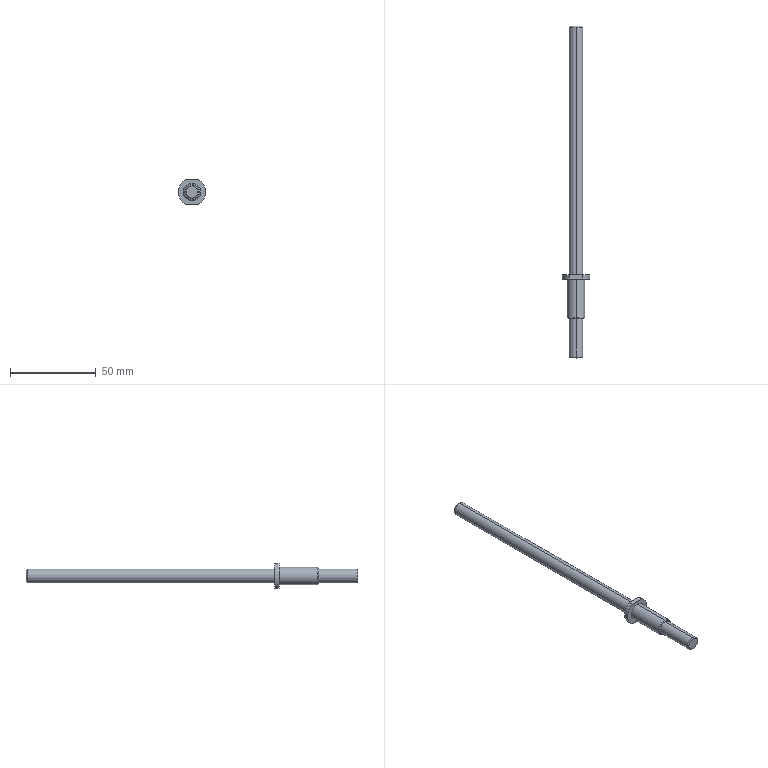Part | STEP file | 11-FG-B04411 | 1 solid | 21 faces | box 16 x 193.5 x 14 mm | volume 10709 mm3 | cylinder 8 | plane 7 | cone 6 | commonest cylinder face diameters 8 x4 10 x2 16 x2
STEP:
#1=CARTESIAN_POINT('',(0.,193.5,3.));
#2=VERTEX_POINT('',#1);
#3=CARTESIAN_POINT('',(0.,193.5,-3.));
#4=VERTEX_POINT('',#3);
#5=CARTESIAN_POINT('',(0.,193.5,0.));
#6=DIRECTION('',(0.,1.,0.));
#7=DIRECTION('',(0.,0.,1.));
#8=AXIS2_PLACEMENT_3D('',#5,#6,#7);
#9=CIRCLE('',#8,3.);
#10=EDGE_CURVE('',#2,#4,#9,.T.);
#11=ORIENTED_EDGE('',*,*,#10,.F.);
#12=CARTESIAN_POINT('',(0.,192.5,4.));
#13=VERTEX_POINT('',#12);
#14=CARTESIAN_POINT('',(0.,192.5,4.));
#15=DIRECTION('',(0.,-0.7071,0.7071));
#16=VECTOR('',#15,1000.);
#17=LINE('',#14,#16);
#18=EDGE_CURVE('',#2,#13,#17,.T.);
#19=ORIENTED_EDGE('',*,*,#18,.T.);
#20=CARTESIAN_POINT('',(0.,192.5,-4.));
#21=VERTEX_POINT('',#20);
#22=CARTESIAN_POINT('',(0.,192.5,0.));
#23=DIRECTION('',(0.,-1.,0.));
#24=DIRECTION('',(0.,0.,1.));
#25=AXIS2_PLACEMENT_3D('',#22,#23,#24);
#26=CIRCLE('',#25,4.);
#27=EDGE_CURVE('',#21,#13,#26,.T.);
#28=ORIENTED_EDGE('',*,*,#27,.F.);
#29=CARTESIAN_POINT('',(0.,192.5,-4.));
#30=DIRECTION('',(0.,-0.7071,-0.7071));
#31=VECTOR('',#30,1000.);
#32=LINE('',#29,#31);
#33=EDGE_CURVE('',#4,#21,#32,.T.);
#34=ORIENTED_EDGE('',*,*,#33,.F.);
#35=EDGE_LOOP('',(#11,#19,#28,#34));
#36=FACE_OUTER_BOUND('',#35,.T.);
#37=CARTESIAN_POINT('',(0.,192.5,0.));
#38=DIRECTION('',(0.,-1.,0.));
#39=DIRECTION('',(0.,0.,-1.));
#40=AXIS2_PLACEMENT_3D('',#37,#38,#39);
#41=CONICAL_SURFACE('',#40,4.,0.7854);
#42=ADVANCED_FACE('',(#36),#41,.T.);
#43=CARTESIAN_POINT('',(0.,23.,-4.5));
#44=VERTEX_POINT('',#43);
#45=CARTESIAN_POINT('',(0.,23.,4.5));
#46=VERTEX_POINT('',#45);
#47=CARTESIAN_POINT('',(0.,23.,0.));
#48=DIRECTION('',(0.,-1.,0.));
#49=DIRECTION('',(0.,0.,-1.));
#50=AXIS2_PLACEMENT_3D('',#47,#48,#49);
#51=CIRCLE('',#50,4.5);
#52=EDGE_CURVE('',#44,#46,#51,.T.);
#53=ORIENTED_EDGE('',*,*,#52,.F.);
#54=CARTESIAN_POINT('',(0.,23.5,-5.));
#55=VERTEX_POINT('',#54);
#56=CARTESIAN_POINT('',(0.,23.,-4.5));
#57=DIRECTION('',(0.,0.7071,-0.7071));
#58=VECTOR('',#57,1000.);
#59=LINE('',#56,#58);
#60=EDGE_CURVE('',#44,#55,#59,.T.);
#61=ORIENTED_EDGE('',*,*,#60,.T.);
#62=CARTESIAN_POINT('',(0.,23.5,5.));
#63=VERTEX_POINT('',#62);
#64=CARTESIAN_POINT('',(0.,23.5,0.));
#65=DIRECTION('',(0.,1.,0.));
#66=DIRECTION('',(0.,0.,-1.));
#67=AXIS2_PLACEMENT_3D('',#64,#65,#66);
#68=CIRCLE('',#67,5.);
#69=EDGE_CURVE('',#63,#55,#68,.T.);
#70=ORIENTED_EDGE('',*,*,#69,.F.);
#71=CARTESIAN_POINT('',(0.,23.,4.5));
#72=DIRECTION('',(0.,0.7071,0.7071));
#73=VECTOR('',#72,1000.);
#74=LINE('',#71,#73);
#75=EDGE_CURVE('',#46,#63,#74,.T.);
#76=ORIENTED_EDGE('',*,*,#75,.F.);
#77=EDGE_LOOP('',(#53,#61,#70,#76));
#78=FACE_OUTER_BOUND('',#77,.T.);
#79=CARTESIAN_POINT('',(0.,23.,0.));
#80=DIRECTION('',(0.,1.,0.));
#81=DIRECTION('',(0.,0.,1.));
#82=AXIS2_PLACEMENT_3D('',#79,#80,#81);
#83=CONICAL_SURFACE('',#82,4.5,0.7854);
#84=ADVANCED_FACE('',(#78),#83,.T.);
#85=CARTESIAN_POINT('',(0.,0.,-3.5));
#86=VERTEX_POINT('',#85);
#87=CARTESIAN_POINT('',(0.,0.,3.5));
#88=VERTEX_POINT('',#87);
#89=CARTESIAN_POINT('',(0.,0.,0.));
#90=DIRECTION('',(0.,-1.,0.));
#91=DIRECTION('',(0.,0.,-1.));
#92=AXIS2_PLACEMENT_3D('',#89,#90,#91);
#93=CIRCLE('',#92,3.5);
#94=EDGE_CURVE('',#86,#88,#93,.T.);
#95=ORIENTED_EDGE('',*,*,#94,.F.);
#96=CARTESIAN_POINT('',(0.,0.5,-4.));
#97=VERTEX_POINT('',#96);
#98=CARTESIAN_POINT('',(0.,0.,-3.5));
#99=DIRECTION('',(0.,0.7071,-0.7071));
#100=VECTOR('',#99,1000.);
#101=LINE('',#98,#100);
#102=EDGE_CURVE('',#86,#97,#101,.T.);
#103=ORIENTED_EDGE('',*,*,#102,.T.);
#104=CARTESIAN_POINT('',(0.,0.5,4.));
#105=VERTEX_POINT('',#104);
#106=CARTESIAN_POINT('',(0.,0.5,0.));
#107=DIRECTION('',(0.,1.,0.));
#108=DIRECTION('',(0.,0.,-1.));
#109=AXIS2_PLACEMENT_3D('',#106,#107,#108);
#110=CIRCLE('',#109,4.);
#111=EDGE_CURVE('',#105,#97,#110,.T.);
#112=ORIENTED_EDGE('',*,*,#111,.F.);
#113=CARTESIAN_POINT('',(0.,0.,3.5));
#114=DIRECTION('',(0.,0.7071,0.7071));
#115=VECTOR('',#114,1000.);
#116=LINE('',#113,#115);
#117=EDGE_CURVE('',#88,#105,#116,.T.);
#118=ORIENTED_EDGE('',*,*,#117,.F.);
#119=EDGE_LOOP('',(#95,#103,#112,#118));
#120=FACE_OUTER_BOUND('',#119,.T.);
#121=CARTESIAN_POINT('',(0.,0.,0.));
#122=DIRECTION('',(0.,1.,0.));
#123=DIRECTION('',(0.,0.,1.));
#124=AXIS2_PLACEMENT_3D('',#121,#122,#123);
#125=CONICAL_SURFACE('',#124,3.5,0.7854);
#126=ADVANCED_FACE('',(#120),#125,.T.);
#127=CARTESIAN_POINT('',(0.,23.,-4.));
#128=VERTEX_POINT('',#127);
#129=CARTESIAN_POINT('',(0.,23.,4.));
#130=VERTEX_POINT('',#129);
#131=CARTESIAN_POINT('',(0.,23.,0.));
#132=DIRECTION('',(0.,-1.,0.));
#133=DIRECTION('',(0.,0.,-1.));
#134=AXIS2_PLACEMENT_3D('',#131,#132,#133);
#135=CIRCLE('',#134,4.);
#136=EDGE_CURVE('',#128,#130,#135,.T.);
#137=ORIENTED_EDGE('',*,*,#136,.T.);
#138=CARTESIAN_POINT('',(0.,0.,4.));
#139=DIRECTION('',(0.,-1.,0.));
#140=VECTOR('',#139,1000.);
#141=LINE('',#138,#140);
#142=EDGE_CURVE('',#130,#105,#141,.T.);
#143=ORIENTED_EDGE('',*,*,#142,.T.);
#144=ORIENTED_EDGE('',*,*,#111,.T.);
#145=CARTESIAN_POINT('',(0.,0.,-4.));
#146=DIRECTION('',(0.,-1.,0.));
#147=VECTOR('',#146,1000.);
#148=LINE('',#145,#147);
#149=EDGE_CURVE('',#128,#97,#148,.T.);
#150=ORIENTED_EDGE('',*,*,#149,.F.);
#151=EDGE_LOOP('',(#137,#143,#144,#150));
#152=FACE_OUTER_BOUND('',#151,.T.);
#153=CARTESIAN_POINT('',(0.,0.,0.));
#154=DIRECTION('',(0.,-1.,0.));
#155=DIRECTION('',(0.,0.,-1.));
#156=AXIS2_PLACEMENT_3D('',#153,#154,#155);
#157=CYLINDRICAL_SURFACE('',#156,4.);
#158=ADVANCED_FACE('',(#152),#157,.T.);
#159=CARTESIAN_POINT('',(0.,46.,-5.));
#160=VERTEX_POINT('',#159);
#161=CARTESIAN_POINT('',(0.,46.,5.));
#162=VERTEX_POINT('',#161);
#163=CARTESIAN_POINT('',(0.,46.,0.));
#164=DIRECTION('',(0.,-1.,0.));
#165=DIRECTION('',(0.,0.,-1.));
#166=AXIS2_PLACEMENT_3D('',#163,#164,#165);
#167=CIRCLE('',#166,5.);
#168=EDGE_CURVE('',#160,#162,#167,.T.);
#169=ORIENTED_EDGE('',*,*,#168,.T.);
#170=CARTESIAN_POINT('',(0.,0.,5.));
#171=DIRECTION('',(0.,-1.,0.));
#172=VECTOR('',#171,1000.);
#173=LINE('',#170,#172);
#174=EDGE_CURVE('',#162,#63,#173,.T.);
#175=ORIENTED_EDGE('',*,*,#174,.T.);
#176=ORIENTED_EDGE('',*,*,#69,.T.);
#177=CARTESIAN_POINT('',(0.,0.,-5.));
#178=DIRECTION('',(0.,-1.,0.));
#179=VECTOR('',#178,1000.);
#180=LINE('',#177,#179);
#181=EDGE_CURVE('',#160,#55,#180,.T.);
#182=ORIENTED_EDGE('',*,*,#181,.F.);
#183=EDGE_LOOP('',(#169,#175,#176,#182));
#184=FACE_OUTER_BOUND('',#183,.T.);
#185=CARTESIAN_POINT('',(0.,0.,0.));
#186=DIRECTION('',(0.,-1.,0.));
#187=DIRECTION('',(0.,0.,-1.));
#188=AXIS2_PLACEMENT_3D('',#185,#186,#187);
#189=CYLINDRICAL_SURFACE('',#188,5.);
#190=ADVANCED_FACE('',(#184),#189,.T.);
#191=ORIENTED_EDGE('',*,*,#27,.T.);
#192=CARTESIAN_POINT('',(0.,48.5,4.));
#193=VERTEX_POINT('',#192);
#194=CARTESIAN_POINT('',(0.,0.,4.));
#195=DIRECTION('',(0.,-1.,0.));
#196=VECTOR('',#195,1000.);
#197=LINE('',#194,#196);
#198=EDGE_CURVE('',#13,#193,#197,.T.);
#199=ORIENTED_EDGE('',*,*,#198,.T.);
#200=CARTESIAN_POINT('',(0.,48.5,-4.));
#201=VERTEX_POINT('',#200);
#202=CARTESIAN_POINT('',(0.,48.5,0.));
#203=DIRECTION('',(0.,-1.,0.));
#204=DIRECTION('',(0.,0.,-1.));
#205=AXIS2_PLACEMENT_3D('',#202,#203,#204);
#206=CIRCLE('',#205,4.);
#207=EDGE_CURVE('',#201,#193,#206,.T.);
#208=ORIENTED_EDGE('',*,*,#207,.F.);
#209=CARTESIAN_POINT('',(0.,0.,-4.));
#210=DIRECTION('',(0.,-1.,0.));
#211=VECTOR('',#210,1000.);
#212=LINE('',#209,#211);
#213=EDGE_CURVE('',#21,#201,#212,.T.);
#214=ORIENTED_EDGE('',*,*,#213,.F.);
#215=EDGE_LOOP('',(#191,#199,#208,#214));
#216=FACE_OUTER_BOUND('',#215,.T.);
#217=CARTESIAN_POINT('',(0.,0.,0.));
#218=DIRECTION('',(0.,-1.,0.));
#219=DIRECTION('',(0.,0.,-1.));
#220=AXIS2_PLACEMENT_3D('',#217,#218,#219);
#221=CYLINDRICAL_SURFACE('',#220,4.);
#222=ADVANCED_FACE('',(#216),#221,.T.);
#223=CARTESIAN_POINT('',(3.873,46.,7.));
#224=VERTEX_POINT('',#223);
#225=CARTESIAN_POINT('',(3.873,48.5,7.));
#226=VERTEX_POINT('',#225);
#227=CARTESIAN_POINT('',(3.873,38.5,7.));
#228=DIRECTION('',(0.,1.,0.));
#229=VECTOR('',#228,1000.);
#230=LINE('',#227,#229);
#231=EDGE_CURVE('',#224,#226,#230,.T.);
#232=ORIENTED_EDGE('',*,*,#231,.F.);
#233=CARTESIAN_POINT('',(3.873,46.,-7.));
#234=VERTEX_POINT('',#233);
#235=CARTESIAN_POINT('',(0.,46.,0.));
#236=DIRECTION('',(0.,-1.,0.));
#237=DIRECTION('',(0.,0.,-1.));
#238=AXIS2_PLACEMENT_3D('',#235,#236,#237);
#239=CIRCLE('',#238,8.);
#240=EDGE_CURVE('',#234,#224,#239,.T.);
#241=ORIENTED_EDGE('',*,*,#240,.F.);
#242=CARTESIAN_POINT('',(3.873,48.5,-7.));
#243=VERTEX_POINT('',#242);
#244=CARTESIAN_POINT('',(3.873,38.5,-7.));
#245=DIRECTION('',(0.,1.,0.));
#246=VECTOR('',#245,1000.);
#247=LINE('',#244,#246);
#248=EDGE_CURVE('',#234,#243,#247,.T.);
#249=ORIENTED_EDGE('',*,*,#248,.T.);
#250=CARTESIAN_POINT('',(0.,48.5,0.));
#251=DIRECTION('',(0.,-1.,0.));
#252=DIRECTION('',(0.,0.,-1.));
#253=AXIS2_PLACEMENT_3D('',#250,#251,#252);
#254=CIRCLE('',#253,8.);
#255=EDGE_CURVE('',#243,#226,#254,.T.);
#256=ORIENTED_EDGE('',*,*,#255,.T.);
#257=EDGE_LOOP('',(#232,#241,#249,#256));
#258=FACE_OUTER_BOUND('',#257,.T.);
#259=CARTESIAN_POINT('',(0.,0.,0.));
#260=DIRECTION('',(0.,-1.,0.));
#261=DIRECTION('',(0.,0.,-1.));
#262=AXIS2_PLACEMENT_3D('',#259,#260,#261);
#263=CYLINDRICAL_SURFACE('',#262,8.);
#264=ADVANCED_FACE('',(#258),#263,.T.);
#265=CARTESIAN_POINT('',(0.,193.5,0.));
#266=DIRECTION('',(0.,1.,0.));
#267=DIRECTION('',(0.,0.,1.));
#268=AXIS2_PLACEMENT_3D('',#265,#266,#267);
#269=CIRCLE('',#268,3.);
#270=EDGE_CURVE('',#4,#2,#269,.T.);
#271=ORIENTED_EDGE('',*,*,#270,.T.);
#272=ORIENTED_EDGE('',*,*,#10,.T.);
#273=EDGE_LOOP('',(#271,#272));
#274=FACE_OUTER_BOUND('',#273,.T.);
#275=CARTESIAN_POINT('',(0.,193.5,0.));
#276=DIRECTION('',(0.,1.,0.));
#277=DIRECTION('',(0.,0.,1.));
#278=AXIS2_PLACEMENT_3D('',#275,#276,#277);
#279=PLANE('',#278);
#280=ADVANCED_FACE('',(#274),#279,.T.);
#281=ORIENTED_EDGE('',*,*,#198,.F.);
#282=CARTESIAN_POINT('',(0.,192.5,0.));
#283=DIRECTION('',(0.,-1.,0.));
#284=DIRECTION('',(0.,0.,1.));
#285=AXIS2_PLACEMENT_3D('',#282,#283,#284);
#286=CIRCLE('',#285,4.);
#287=EDGE_CURVE('',#13,#21,#286,.T.);
#288=ORIENTED_EDGE('',*,*,#287,.T.);
#289=ORIENTED_EDGE('',*,*,#213,.T.);
#290=CARTESIAN_POINT('',(0.,48.5,0.));
#291=DIRECTION('',(0.,-1.,0.));
#292=DIRECTION('',(0.,0.,-1.));
#293=AXIS2_PLACEMENT_3D('',#290,#291,#292);
#294=CIRCLE('',#293,4.);
#295=EDGE_CURVE('',#193,#201,#294,.T.);
#296=ORIENTED_EDGE('',*,*,#295,.F.);
#297=EDGE_LOOP('',(#281,#288,#289,#296));
#298=FACE_OUTER_BOUND('',#297,.T.);
#299=CARTESIAN_POINT('',(0.,0.,0.));
#300=DIRECTION('',(0.,-1.,0.));
#301=DIRECTION('',(0.,0.,-1.));
#302=AXIS2_PLACEMENT_3D('',#299,#300,#301);
#303=CYLINDRICAL_SURFACE('',#302,4.);
#304=ADVANCED_FACE('',(#298),#303,.T.);
#305=CARTESIAN_POINT('',(-3.873,48.5,7.));
#306=VERTEX_POINT('',#305);
#307=CARTESIAN_POINT('',(-3.873,48.5,7.));
#308=DIRECTION('',(-1.,0.,0.));
#309=VECTOR('',#308,1000.);
#310=LINE('',#307,#309);
#311=EDGE_CURVE('',#226,#306,#310,.T.);
#312=ORIENTED_EDGE('',*,*,#311,.F.);
#313=ORIENTED_EDGE('',*,*,#255,.F.);
#314=CARTESIAN_POINT('',(-3.873,48.5,-7.));
#315=VERTEX_POINT('',#314);
#316=CARTESIAN_POINT('',(-3.873,48.5,-7.));
#317=DIRECTION('',(1.,0.,0.));
#318=VECTOR('',#317,1000.);
#319=LINE('',#316,#318);
#320=EDGE_CURVE('',#315,#243,#319,.T.);
#321=ORIENTED_EDGE('',*,*,#320,.F.);
#322=CARTESIAN_POINT('',(0.,48.5,0.));
#323=DIRECTION('',(0.,-1.,0.));
#324=DIRECTION('',(0.,0.,-1.));
#325=AXIS2_PLACEMENT_3D('',#322,#323,#324);
#326=CIRCLE('',#325,8.);
#327=EDGE_CURVE('',#306,#315,#326,.T.);
#328=ORIENTED_EDGE('',*,*,#327,.F.);
#329=EDGE_LOOP('',(#312,#313,#321,#328));
#330=FACE_OUTER_BOUND('',#329,.T.);
#331=ORIENTED_EDGE('',*,*,#207,.T.);
#332=ORIENTED_EDGE('',*,*,#295,.T.);
#333=EDGE_LOOP('',(#331,#332));
#334=FACE_BOUND('',#333,.T.);
#335=CARTESIAN_POINT('',(4.,48.5,0.));
#336=DIRECTION('',(0.,1.,0.));
#337=DIRECTION('',(0.,0.,1.));
#338=AXIS2_PLACEMENT_3D('',#335,#336,#337);
#339=PLANE('',#338);
#340=ADVANCED_FACE('',(#330,#334),#339,.T.);
#341=CARTESIAN_POINT('',(-3.873,46.,7.));
#342=VERTEX_POINT('',#341);
#343=CARTESIAN_POINT('',(-3.873,38.5,7.));
#344=DIRECTION('',(0.,1.,0.));
#345=VECTOR('',#344,1000.);
#346=LINE('',#343,#345);
#347=EDGE_CURVE('',#342,#306,#346,.T.);
#348=ORIENTED_EDGE('',*,*,#347,.T.);
#349=ORIENTED_EDGE('',*,*,#327,.T.);
#350=CARTESIAN_POINT('',(-3.873,46.,-7.));
#351=VERTEX_POINT('',#350);
#352=CARTESIAN_POINT('',(-3.873,38.5,-7.));
#353=DIRECTION('',(0.,1.,0.));
#354=VECTOR('',#353,1000.);
#355=LINE('',#352,#354);
#356=EDGE_CURVE('',#351,#315,#355,.T.);
#357=ORIENTED_EDGE('',*,*,#356,.F.);
#358=CARTESIAN_POINT('',(0.,46.,0.));
#359=DIRECTION('',(0.,-1.,0.));
#360=DIRECTION('',(0.,0.,-1.));
#361=AXIS2_PLACEMENT_3D('',#358,#359,#360);
#362=CIRCLE('',#361,8.);
#363=EDGE_CURVE('',#342,#351,#362,.T.);
#364=ORIENTED_EDGE('',*,*,#363,.F.);
#365=EDGE_LOOP('',(#348,#349,#357,#364));
#366=FACE_OUTER_BOUND('',#365,.T.);
#367=CARTESIAN_POINT('',(0.,0.,0.));
#368=DIRECTION('',(0.,-1.,0.));
#369=DIRECTION('',(0.,0.,-1.));
#370=AXIS2_PLACEMENT_3D('',#367,#368,#369);
#371=CYLINDRICAL_SURFACE('',#370,8.);
#372=ADVANCED_FACE('',(#366),#371,.T.);
#373=CARTESIAN_POINT('',(8.,46.,7.));
#374=DIRECTION('',(1.,0.,0.));
#375=VECTOR('',#374,1000.);
#376=LINE('',#373,#375);
#377=EDGE_CURVE('',#342,#224,#376,.T.);
#378=ORIENTED_EDGE('',*,*,#377,.F.);
#379=ORIENTED_EDGE('',*,*,#363,.T.);
#380=CARTESIAN_POINT('',(8.,46.,-7.));
#381=DIRECTION('',(-1.,0.,0.));
#382=VECTOR('',#381,1000.);
#383=LINE('',#380,#382);
#384=EDGE_CURVE('',#234,#351,#383,.T.);
#385=ORIENTED_EDGE('',*,*,#384,.F.);
#386=ORIENTED_EDGE('',*,*,#240,.T.);
#387=EDGE_LOOP('',(#378,#379,#385,#386));
#388=FACE_OUTER_BOUND('',#387,.T.);
#389=ORIENTED_EDGE('',*,*,#168,.F.);
#390=CARTESIAN_POINT('',(0.,46.,0.));
#391=DIRECTION('',(0.,-1.,0.));
#392=DIRECTION('',(0.,0.,-1.));
#393=AXIS2_PLACEMENT_3D('',#390,#391,#392);
#394=CIRCLE('',#393,5.);
#395=EDGE_CURVE('',#162,#160,#394,.T.);
#396=ORIENTED_EDGE('',*,*,#395,.F.);
#397=EDGE_LOOP('',(#389,#396));
#398=FACE_BOUND('',#397,.T.);
#399=CARTESIAN_POINT('',(8.,46.,0.));
#400=DIRECTION('',(0.,-1.,0.));
#401=DIRECTION('',(0.,0.,-1.));
#402=AXIS2_PLACEMENT_3D('',#399,#400,#401);
#403=PLANE('',#402);
#404=ADVANCED_FACE('',(#388,#398),#403,.T.);
#405=ORIENTED_EDGE('',*,*,#174,.F.);
#406=ORIENTED_EDGE('',*,*,#395,.T.);
#407=ORIENTED_EDGE('',*,*,#181,.T.);
#408=CARTESIAN_POINT('',(0.,23.5,0.));
#409=DIRECTION('',(0.,1.,0.));
#410=DIRECTION('',(0.,0.,-1.));
#411=AXIS2_PLACEMENT_3D('',#408,#409,#410);
#412=CIRCLE('',#411,5.);
#413=EDGE_CURVE('',#55,#63,#412,.T.);
#414=ORIENTED_EDGE('',*,*,#413,.T.);
#415=EDGE_LOOP('',(#405,#406,#407,#414));
#416=FACE_OUTER_BOUND('',#415,.T.);
#417=CARTESIAN_POINT('',(0.,0.,0.));
#418=DIRECTION('',(0.,-1.,0.));
#419=DIRECTION('',(0.,0.,-1.));
#420=AXIS2_PLACEMENT_3D('',#417,#418,#419);
#421=CYLINDRICAL_SURFACE('',#420,5.);
#422=ADVANCED_FACE('',(#416),#421,.T.);
#423=CARTESIAN_POINT('',(0.,23.,0.));
#424=DIRECTION('',(0.,-1.,0.));
#425=DIRECTION('',(0.,0.,-1.));
#426=AXIS2_PLACEMENT_3D('',#423,#424,#425);
#427=CIRCLE('',#426,4.5);
#428=EDGE_CURVE('',#46,#44,#427,.T.);
#429=ORIENTED_EDGE('',*,*,#428,.T.);
#430=ORIENTED_EDGE('',*,*,#52,.T.);
#431=EDGE_LOOP('',(#429,#430));
#432=FACE_OUTER_BOUND('',#431,.T.);
#433=ORIENTED_EDGE('',*,*,#136,.F.);
#434=CARTESIAN_POINT('',(0.,23.,0.));
#435=DIRECTION('',(0.,-1.,0.));
#436=DIRECTION('',(0.,0.,-1.));
#437=AXIS2_PLACEMENT_3D('',#434,#435,#436);
#438=CIRCLE('',#437,4.);
#439=EDGE_CURVE('',#130,#128,#438,.T.);
#440=ORIENTED_EDGE('',*,*,#439,.F.);
#441=EDGE_LOOP('',(#433,#440));
#442=FACE_BOUND('',#441,.T.);
#443=CARTESIAN_POINT('',(5.,23.,0.));
#444=DIRECTION('',(0.,-1.,0.));
#445=DIRECTION('',(0.,0.,-1.));
#446=AXIS2_PLACEMENT_3D('',#443,#444,#445);
#447=PLANE('',#446);
#448=ADVANCED_FACE('',(#432,#442),#447,.T.);
#449=ORIENTED_EDGE('',*,*,#142,.F.);
#450=ORIENTED_EDGE('',*,*,#439,.T.);
#451=ORIENTED_EDGE('',*,*,#149,.T.);
#452=CARTESIAN_POINT('',(0.,0.5,0.));
#453=DIRECTION('',(0.,1.,0.));
#454=DIRECTION('',(0.,0.,-1.));
#455=AXIS2_PLACEMENT_3D('',#452,#453,#454);
#456=CIRCLE('',#455,4.);
#457=EDGE_CURVE('',#97,#105,#456,.T.);
#458=ORIENTED_EDGE('',*,*,#457,.T.);
#459=EDGE_LOOP('',(#449,#450,#451,#458));
#460=FACE_OUTER_BOUND('',#459,.T.);
#461=CARTESIAN_POINT('',(0.,0.,0.));
#462=DIRECTION('',(0.,-1.,0.));
#463=DIRECTION('',(0.,0.,-1.));
#464=AXIS2_PLACEMENT_3D('',#461,#462,#463);
#465=CYLINDRICAL_SURFACE('',#464,4.);
#466=ADVANCED_FACE('',(#460),#465,.T.);
#467=CARTESIAN_POINT('',(0.,0.,0.));
#468=DIRECTION('',(0.,-1.,0.));
#469=DIRECTION('',(0.,0.,-1.));
#470=AXIS2_PLACEMENT_3D('',#467,#468,#469);
#471=CIRCLE('',#470,3.5);
#472=EDGE_CURVE('',#88,#86,#471,.T.);
#473=ORIENTED_EDGE('',*,*,#472,.T.);
#474=ORIENTED_EDGE('',*,*,#94,.T.);
#475=EDGE_LOOP('',(#473,#474));
#476=FACE_OUTER_BOUND('',#475,.T.);
#477=CARTESIAN_POINT('',(4.,0.,0.));
#478=DIRECTION('',(0.,-1.,0.));
#479=DIRECTION('',(0.,0.,-1.));
#480=AXIS2_PLACEMENT_3D('',#477,#478,#479);
#481=PLANE('',#480);
#482=ADVANCED_FACE('',(#476),#481,.T.);
#483=ORIENTED_EDGE('',*,*,#102,.F.);
#484=ORIENTED_EDGE('',*,*,#472,.F.);
#485=ORIENTED_EDGE('',*,*,#117,.T.);
#486=ORIENTED_EDGE('',*,*,#457,.F.);
#487=EDGE_LOOP('',(#483,#484,#485,#486));
#488=FACE_OUTER_BOUND('',#487,.T.);
#489=CARTESIAN_POINT('',(0.,0.,0.));
#490=DIRECTION('',(0.,1.,0.));
#491=DIRECTION('',(0.,0.,1.));
#492=AXIS2_PLACEMENT_3D('',#489,#490,#491);
#493=CONICAL_SURFACE('',#492,3.5,0.7854);
#494=ADVANCED_FACE('',(#488),#493,.T.);
#495=ORIENTED_EDGE('',*,*,#60,.F.);
#496=ORIENTED_EDGE('',*,*,#428,.F.);
#497=ORIENTED_EDGE('',*,*,#75,.T.);
#498=ORIENTED_EDGE('',*,*,#413,.F.);
#499=EDGE_LOOP('',(#495,#496,#497,#498));
#500=FACE_OUTER_BOUND('',#499,.T.);
#501=CARTESIAN_POINT('',(0.,23.,0.));
#502=DIRECTION('',(0.,1.,0.));
#503=DIRECTION('',(0.,0.,1.));
#504=AXIS2_PLACEMENT_3D('',#501,#502,#503);
#505=CONICAL_SURFACE('',#504,4.5,0.7854);
#506=ADVANCED_FACE('',(#500),#505,.T.);
#507=ORIENTED_EDGE('',*,*,#18,.F.);
#508=ORIENTED_EDGE('',*,*,#270,.F.);
#509=ORIENTED_EDGE('',*,*,#33,.T.);
#510=ORIENTED_EDGE('',*,*,#287,.F.);
#511=EDGE_LOOP('',(#507,#508,#509,#510));
#512=FACE_OUTER_BOUND('',#511,.T.);
#513=CARTESIAN_POINT('',(0.,192.5,0.));
#514=DIRECTION('',(0.,-1.,0.));
#515=DIRECTION('',(0.,0.,-1.));
#516=AXIS2_PLACEMENT_3D('',#513,#514,#515);
#517=CONICAL_SURFACE('',#516,4.,0.7854);
#518=ADVANCED_FACE('',(#512),#517,.T.);
#519=ORIENTED_EDGE('',*,*,#384,.T.);
#520=ORIENTED_EDGE('',*,*,#356,.T.);
#521=ORIENTED_EDGE('',*,*,#320,.T.);
#522=ORIENTED_EDGE('',*,*,#248,.F.);
#523=EDGE_LOOP('',(#519,#520,#521,#522));
#524=FACE_OUTER_BOUND('',#523,.T.);
#525=CARTESIAN_POINT('',(-3.873,38.5,-7.));
#526=DIRECTION('',(0.,0.,1.));
#527=DIRECTION('',(1.,0.,0.));
#528=AXIS2_PLACEMENT_3D('',#525,#526,#527);
#529=PLANE('',#528);
#530=ADVANCED_FACE('',(#524),#529,.F.);
#531=ORIENTED_EDGE('',*,*,#377,.T.);
#532=ORIENTED_EDGE('',*,*,#231,.T.);
#533=ORIENTED_EDGE('',*,*,#311,.T.);
#534=ORIENTED_EDGE('',*,*,#347,.F.);
#535=EDGE_LOOP('',(#531,#532,#533,#534));
#536=FACE_OUTER_BOUND('',#535,.T.);
#537=CARTESIAN_POINT('',(-3.873,38.5,7.));
#538=DIRECTION('',(0.,0.,-1.));
#539=DIRECTION('',(-1.,0.,0.));
#540=AXIS2_PLACEMENT_3D('',#537,#538,#539);
#541=PLANE('',#540);
#542=ADVANCED_FACE('',(#536),#541,.F.);
#543=CLOSED_SHELL('',(#42,#84,#126,#158,#190,#222,#264,#280,#304,#340,#372,#404,#422,#448,#466,#482,#494,#506,#518,#530,#542));
#544=MANIFOLD_SOLID_BREP('',#543);
#545=CARTESIAN_POINT('',(0.,0.,0.));
#546=DIRECTION('',(0.,0.,1.));
#547=DIRECTION('',(1.,0.,0.));
#548=AXIS2_PLACEMENT_3D('',#545,#546,#547);
#549=(LENGTH_UNIT()NAMED_UNIT(*)SI_UNIT(.MILLI.,.METRE.));
#550=UNCERTAINTY_MEASURE_WITH_UNIT(LENGTH_MEASURE(0.00001),#549,'','');
#551=(NAMED_UNIT(*)PLANE_ANGLE_UNIT()SI_UNIT($,.RADIAN.));
#552=(NAMED_UNIT(*)SI_UNIT($,.STERADIAN.)SOLID_ANGLE_UNIT());
#553=(GEOMETRIC_REPRESENTATION_CONTEXT(3)GLOBAL_UNCERTAINTY_ASSIGNED_CONTEXT((#550))GLOBAL_UNIT_ASSIGNED_CONTEXT((#549,#551,#552))REPRESENTATION_CONTEXT('',''));
#554=ADVANCED_BREP_SHAPE_REPRESENTATION('',(#544,#548),#553);